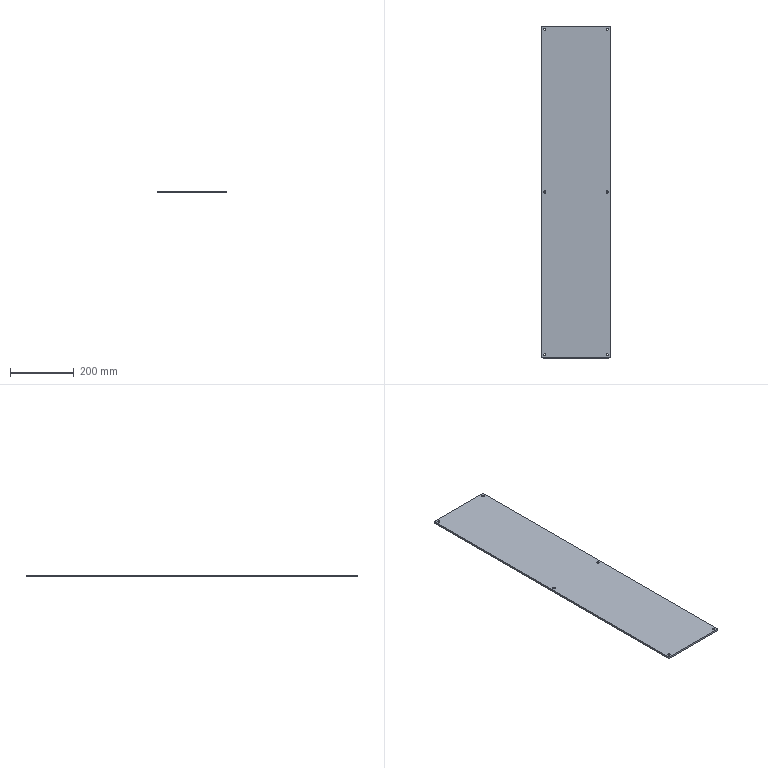Part | SolidWorks | features Extrusion 1, Fillet 1, HoleWzd 1 | 1 solid | 22 faces | box 215 x 1038 x 6 mm | volume 1337506 mm3 | cylinder 16 | plane 6 | commonest cylinder face diameters 7 x12 10 x4
STEP:
#1=CARTESIAN_POINT('',(101.,509.,6.));
#2=VERTEX_POINT('',#1);
#3=CARTESIAN_POINT('',(94.,509.,6.));
#4=VERTEX_POINT('',#3);
#5=CARTESIAN_POINT('',(97.5,509.,6.));
#6=DIRECTION('',(0.,0.,-1.));
#7=DIRECTION('',(-1.,0.,0.));
#8=AXIS2_PLACEMENT_3D('',#5,#6,#7);
#9=CIRCLE('',#8,3.5);
#10=EDGE_CURVE('',#2,#4,#9,.T.);
#11=ORIENTED_EDGE('',*,*,#10,.F.);
#12=CARTESIAN_POINT('',(101.,509.,0.));
#13=VERTEX_POINT('',#12);
#14=CARTESIAN_POINT('',(101.,509.,0.));
#15=DIRECTION('',(0.,0.,-1.));
#16=VECTOR('',#15,1000.);
#17=LINE('',#14,#16);
#18=EDGE_CURVE('',#2,#13,#17,.T.);
#19=ORIENTED_EDGE('',*,*,#18,.T.);
#20=CARTESIAN_POINT('',(94.,509.,0.));
#21=VERTEX_POINT('',#20);
#22=CARTESIAN_POINT('',(97.5,509.,0.));
#23=DIRECTION('',(0.,0.,-1.));
#24=DIRECTION('',(-1.,0.,0.));
#25=AXIS2_PLACEMENT_3D('',#22,#23,#24);
#26=CIRCLE('',#25,3.5);
#27=EDGE_CURVE('',#13,#21,#26,.T.);
#28=ORIENTED_EDGE('',*,*,#27,.T.);
#29=CARTESIAN_POINT('',(94.,509.,0.));
#30=DIRECTION('',(0.,0.,-1.));
#31=VECTOR('',#30,1000.);
#32=LINE('',#29,#31);
#33=EDGE_CURVE('',#4,#21,#32,.T.);
#34=ORIENTED_EDGE('',*,*,#33,.F.);
#35=EDGE_LOOP('',(#11,#19,#28,#34));
#36=FACE_OUTER_BOUND('',#35,.T.);
#37=CARTESIAN_POINT('',(97.5,509.,0.));
#38=DIRECTION('',(0.,0.,-1.));
#39=DIRECTION('',(-1.,0.,0.));
#40=AXIS2_PLACEMENT_3D('',#37,#38,#39);
#41=CYLINDRICAL_SURFACE('',#40,3.5);
#42=ADVANCED_FACE('',(#36),#41,.F.);
#43=CARTESIAN_POINT('',(101.,-509.,6.));
#44=VERTEX_POINT('',#43);
#45=CARTESIAN_POINT('',(94.,-509.,6.));
#46=VERTEX_POINT('',#45);
#47=CARTESIAN_POINT('',(97.5,-509.,6.));
#48=DIRECTION('',(0.,0.,-1.));
#49=DIRECTION('',(-1.,0.,0.));
#50=AXIS2_PLACEMENT_3D('',#47,#48,#49);
#51=CIRCLE('',#50,3.5);
#52=EDGE_CURVE('',#44,#46,#51,.T.);
#53=ORIENTED_EDGE('',*,*,#52,.F.);
#54=CARTESIAN_POINT('',(101.,-509.,0.));
#55=VERTEX_POINT('',#54);
#56=CARTESIAN_POINT('',(101.,-509.,0.));
#57=DIRECTION('',(0.,0.,-1.));
#58=VECTOR('',#57,1000.);
#59=LINE('',#56,#58);
#60=EDGE_CURVE('',#44,#55,#59,.T.);
#61=ORIENTED_EDGE('',*,*,#60,.T.);
#62=CARTESIAN_POINT('',(94.,-509.,0.));
#63=VERTEX_POINT('',#62);
#64=CARTESIAN_POINT('',(97.5,-509.,0.));
#65=DIRECTION('',(0.,0.,-1.));
#66=DIRECTION('',(-1.,0.,0.));
#67=AXIS2_PLACEMENT_3D('',#64,#65,#66);
#68=CIRCLE('',#67,3.5);
#69=EDGE_CURVE('',#55,#63,#68,.T.);
#70=ORIENTED_EDGE('',*,*,#69,.T.);
#71=CARTESIAN_POINT('',(94.,-509.,0.));
#72=DIRECTION('',(0.,0.,-1.));
#73=VECTOR('',#72,1000.);
#74=LINE('',#71,#73);
#75=EDGE_CURVE('',#46,#63,#74,.T.);
#76=ORIENTED_EDGE('',*,*,#75,.F.);
#77=EDGE_LOOP('',(#53,#61,#70,#76));
#78=FACE_OUTER_BOUND('',#77,.T.);
#79=CARTESIAN_POINT('',(97.5,-509.,0.));
#80=DIRECTION('',(0.,0.,-1.));
#81=DIRECTION('',(-1.,0.,0.));
#82=AXIS2_PLACEMENT_3D('',#79,#80,#81);
#83=CYLINDRICAL_SURFACE('',#82,3.5);
#84=ADVANCED_FACE('',(#78),#83,.F.);
#85=CARTESIAN_POINT('',(-94.,509.,6.));
#86=VERTEX_POINT('',#85);
#87=CARTESIAN_POINT('',(-101.,509.,6.));
#88=VERTEX_POINT('',#87);
#89=CARTESIAN_POINT('',(-97.5,509.,6.));
#90=DIRECTION('',(0.,0.,-1.));
#91=DIRECTION('',(-1.,0.,0.));
#92=AXIS2_PLACEMENT_3D('',#89,#90,#91);
#93=CIRCLE('',#92,3.5);
#94=EDGE_CURVE('',#86,#88,#93,.T.);
#95=ORIENTED_EDGE('',*,*,#94,.F.);
#96=CARTESIAN_POINT('',(-94.,509.,0.));
#97=VERTEX_POINT('',#96);
#98=CARTESIAN_POINT('',(-94.,509.,0.));
#99=DIRECTION('',(0.,0.,-1.));
#100=VECTOR('',#99,1000.);
#101=LINE('',#98,#100);
#102=EDGE_CURVE('',#86,#97,#101,.T.);
#103=ORIENTED_EDGE('',*,*,#102,.T.);
#104=CARTESIAN_POINT('',(-101.,509.,0.));
#105=VERTEX_POINT('',#104);
#106=CARTESIAN_POINT('',(-97.5,509.,0.));
#107=DIRECTION('',(0.,0.,-1.));
#108=DIRECTION('',(-1.,0.,0.));
#109=AXIS2_PLACEMENT_3D('',#106,#107,#108);
#110=CIRCLE('',#109,3.5);
#111=EDGE_CURVE('',#97,#105,#110,.T.);
#112=ORIENTED_EDGE('',*,*,#111,.T.);
#113=CARTESIAN_POINT('',(-101.,509.,0.));
#114=DIRECTION('',(0.,0.,-1.));
#115=VECTOR('',#114,1000.);
#116=LINE('',#113,#115);
#117=EDGE_CURVE('',#88,#105,#116,.T.);
#118=ORIENTED_EDGE('',*,*,#117,.F.);
#119=EDGE_LOOP('',(#95,#103,#112,#118));
#120=FACE_OUTER_BOUND('',#119,.T.);
#121=CARTESIAN_POINT('',(-97.5,509.,0.));
#122=DIRECTION('',(0.,0.,-1.));
#123=DIRECTION('',(-1.,0.,0.));
#124=AXIS2_PLACEMENT_3D('',#121,#122,#123);
#125=CYLINDRICAL_SURFACE('',#124,3.5);
#126=ADVANCED_FACE('',(#120),#125,.F.);
#127=CARTESIAN_POINT('',(-94.,-509.,6.));
#128=VERTEX_POINT('',#127);
#129=CARTESIAN_POINT('',(-101.,-509.,6.));
#130=VERTEX_POINT('',#129);
#131=CARTESIAN_POINT('',(-97.5,-509.,6.));
#132=DIRECTION('',(0.,0.,-1.));
#133=DIRECTION('',(-1.,0.,0.));
#134=AXIS2_PLACEMENT_3D('',#131,#132,#133);
#135=CIRCLE('',#134,3.5);
#136=EDGE_CURVE('',#128,#130,#135,.T.);
#137=ORIENTED_EDGE('',*,*,#136,.F.);
#138=CARTESIAN_POINT('',(-94.,-509.,0.));
#139=VERTEX_POINT('',#138);
#140=CARTESIAN_POINT('',(-94.,-509.,0.));
#141=DIRECTION('',(0.,0.,-1.));
#142=VECTOR('',#141,1000.);
#143=LINE('',#140,#142);
#144=EDGE_CURVE('',#128,#139,#143,.T.);
#145=ORIENTED_EDGE('',*,*,#144,.T.);
#146=CARTESIAN_POINT('',(-101.,-509.,0.));
#147=VERTEX_POINT('',#146);
#148=CARTESIAN_POINT('',(-97.5,-509.,0.));
#149=DIRECTION('',(0.,0.,-1.));
#150=DIRECTION('',(-1.,0.,0.));
#151=AXIS2_PLACEMENT_3D('',#148,#149,#150);
#152=CIRCLE('',#151,3.5);
#153=EDGE_CURVE('',#139,#147,#152,.T.);
#154=ORIENTED_EDGE('',*,*,#153,.T.);
#155=CARTESIAN_POINT('',(-101.,-509.,0.));
#156=DIRECTION('',(0.,0.,-1.));
#157=VECTOR('',#156,1000.);
#158=LINE('',#155,#157);
#159=EDGE_CURVE('',#130,#147,#158,.T.);
#160=ORIENTED_EDGE('',*,*,#159,.F.);
#161=EDGE_LOOP('',(#137,#145,#154,#160));
#162=FACE_OUTER_BOUND('',#161,.T.);
#163=CARTESIAN_POINT('',(-97.5,-509.,0.));
#164=DIRECTION('',(0.,0.,-1.));
#165=DIRECTION('',(-1.,0.,0.));
#166=AXIS2_PLACEMENT_3D('',#163,#164,#165);
#167=CYLINDRICAL_SURFACE('',#166,3.5);
#168=ADVANCED_FACE('',(#162),#167,.F.);
#169=CARTESIAN_POINT('',(101.,0.,6.));
#170=VERTEX_POINT('',#169);
#171=CARTESIAN_POINT('',(94.,0.,6.));
#172=VERTEX_POINT('',#171);
#173=CARTESIAN_POINT('',(97.5,0.,6.));
#174=DIRECTION('',(0.,0.,-1.));
#175=DIRECTION('',(-1.,0.,0.));
#176=AXIS2_PLACEMENT_3D('',#173,#174,#175);
#177=CIRCLE('',#176,3.5);
#178=EDGE_CURVE('',#170,#172,#177,.T.);
#179=ORIENTED_EDGE('',*,*,#178,.F.);
#180=CARTESIAN_POINT('',(101.,0.,0.));
#181=VERTEX_POINT('',#180);
#182=CARTESIAN_POINT('',(101.,0.,0.));
#183=DIRECTION('',(0.,0.,-1.));
#184=VECTOR('',#183,1000.);
#185=LINE('',#182,#184);
#186=EDGE_CURVE('',#170,#181,#185,.T.);
#187=ORIENTED_EDGE('',*,*,#186,.T.);
#188=CARTESIAN_POINT('',(94.,0.,0.));
#189=VERTEX_POINT('',#188);
#190=CARTESIAN_POINT('',(97.5,0.,0.));
#191=DIRECTION('',(0.,0.,-1.));
#192=DIRECTION('',(-1.,0.,0.));
#193=AXIS2_PLACEMENT_3D('',#190,#191,#192);
#194=CIRCLE('',#193,3.5);
#195=EDGE_CURVE('',#181,#189,#194,.T.);
#196=ORIENTED_EDGE('',*,*,#195,.T.);
#197=CARTESIAN_POINT('',(94.,0.,0.));
#198=DIRECTION('',(0.,0.,-1.));
#199=VECTOR('',#198,1000.);
#200=LINE('',#197,#199);
#201=EDGE_CURVE('',#172,#189,#200,.T.);
#202=ORIENTED_EDGE('',*,*,#201,.F.);
#203=EDGE_LOOP('',(#179,#187,#196,#202));
#204=FACE_OUTER_BOUND('',#203,.T.);
#205=CARTESIAN_POINT('',(97.5,0.,0.));
#206=DIRECTION('',(0.,0.,-1.));
#207=DIRECTION('',(-1.,0.,0.));
#208=AXIS2_PLACEMENT_3D('',#205,#206,#207);
#209=CYLINDRICAL_SURFACE('',#208,3.5);
#210=ADVANCED_FACE('',(#204),#209,.F.);
#211=CARTESIAN_POINT('',(-94.,0.,6.));
#212=VERTEX_POINT('',#211);
#213=CARTESIAN_POINT('',(-101.,0.,6.));
#214=VERTEX_POINT('',#213);
#215=CARTESIAN_POINT('',(-97.5,0.,6.));
#216=DIRECTION('',(0.,0.,-1.));
#217=DIRECTION('',(-1.,0.,0.));
#218=AXIS2_PLACEMENT_3D('',#215,#216,#217);
#219=CIRCLE('',#218,3.5);
#220=EDGE_CURVE('',#212,#214,#219,.T.);
#221=ORIENTED_EDGE('',*,*,#220,.F.);
#222=CARTESIAN_POINT('',(-94.,0.,0.));
#223=VERTEX_POINT('',#222);
#224=CARTESIAN_POINT('',(-94.,0.,0.));
#225=DIRECTION('',(0.,0.,-1.));
#226=VECTOR('',#225,1000.);
#227=LINE('',#224,#226);
#228=EDGE_CURVE('',#212,#223,#227,.T.);
#229=ORIENTED_EDGE('',*,*,#228,.T.);
#230=CARTESIAN_POINT('',(-101.,0.,0.));
#231=VERTEX_POINT('',#230);
#232=CARTESIAN_POINT('',(-97.5,0.,0.));
#233=DIRECTION('',(0.,0.,-1.));
#234=DIRECTION('',(-1.,0.,0.));
#235=AXIS2_PLACEMENT_3D('',#232,#233,#234);
#236=CIRCLE('',#235,3.5);
#237=EDGE_CURVE('',#223,#231,#236,.T.);
#238=ORIENTED_EDGE('',*,*,#237,.T.);
#239=CARTESIAN_POINT('',(-101.,0.,0.));
#240=DIRECTION('',(0.,0.,-1.));
#241=VECTOR('',#240,1000.);
#242=LINE('',#239,#241);
#243=EDGE_CURVE('',#214,#231,#242,.T.);
#244=ORIENTED_EDGE('',*,*,#243,.F.);
#245=EDGE_LOOP('',(#221,#229,#238,#244));
#246=FACE_OUTER_BOUND('',#245,.T.);
#247=CARTESIAN_POINT('',(-97.5,0.,0.));
#248=DIRECTION('',(0.,0.,-1.));
#249=DIRECTION('',(-1.,0.,0.));
#250=AXIS2_PLACEMENT_3D('',#247,#248,#249);
#251=CYLINDRICAL_SURFACE('',#250,3.5);
#252=ADVANCED_FACE('',(#246),#251,.F.);
#253=CARTESIAN_POINT('',(107.5,-514.,6.));
#254=VERTEX_POINT('',#253);
#255=CARTESIAN_POINT('',(107.5,514.,6.));
#256=VERTEX_POINT('',#255);
#257=CARTESIAN_POINT('',(107.5,519.,6.));
#258=DIRECTION('',(0.,1.,0.));
#259=VECTOR('',#258,1000.);
#260=LINE('',#257,#259);
#261=EDGE_CURVE('',#254,#256,#260,.T.);
#262=ORIENTED_EDGE('',*,*,#261,.F.);
#263=CARTESIAN_POINT('',(107.5,-514.,0.));
#264=VERTEX_POINT('',#263);
#265=CARTESIAN_POINT('',(107.5,-514.,6.));
#266=DIRECTION('',(0.,0.,-1.));
#267=VECTOR('',#266,1000.);
#268=LINE('',#265,#267);
#269=EDGE_CURVE('',#254,#264,#268,.T.);
#270=ORIENTED_EDGE('',*,*,#269,.T.);
#271=CARTESIAN_POINT('',(107.5,514.,0.));
#272=VERTEX_POINT('',#271);
#273=CARTESIAN_POINT('',(107.5,519.,0.));
#274=DIRECTION('',(0.,1.,0.));
#275=VECTOR('',#274,1000.);
#276=LINE('',#273,#275);
#277=EDGE_CURVE('',#264,#272,#276,.T.);
#278=ORIENTED_EDGE('',*,*,#277,.T.);
#279=CARTESIAN_POINT('',(107.5,514.,6.));
#280=DIRECTION('',(0.,0.,1.));
#281=VECTOR('',#280,1000.);
#282=LINE('',#279,#281);
#283=EDGE_CURVE('',#272,#256,#282,.T.);
#284=ORIENTED_EDGE('',*,*,#283,.T.);
#285=EDGE_LOOP('',(#262,#270,#278,#284));
#286=FACE_OUTER_BOUND('',#285,.T.);
#287=CARTESIAN_POINT('',(107.5,519.,6.));
#288=DIRECTION('',(-1.,0.,0.));
#289=DIRECTION('',(0.,-1.,0.));
#290=AXIS2_PLACEMENT_3D('',#287,#288,#289);
#291=PLANE('',#290);
#292=ADVANCED_FACE('',(#286),#291,.F.);
#293=CARTESIAN_POINT('',(102.5,519.,0.));
#294=VERTEX_POINT('',#293);
#295=CARTESIAN_POINT('',(-102.5,519.,0.));
#296=VERTEX_POINT('',#295);
#297=CARTESIAN_POINT('',(-107.5,519.,0.));
#298=DIRECTION('',(-1.,0.,0.));
#299=VECTOR('',#298,1000.);
#300=LINE('',#297,#299);
#301=EDGE_CURVE('',#294,#296,#300,.T.);
#302=ORIENTED_EDGE('',*,*,#301,.T.);
#303=CARTESIAN_POINT('',(-102.5,519.,6.));
#304=VERTEX_POINT('',#303);
#305=CARTESIAN_POINT('',(-102.5,519.,6.));
#306=DIRECTION('',(0.,0.,1.));
#307=VECTOR('',#306,1000.);
#308=LINE('',#305,#307);
#309=EDGE_CURVE('',#296,#304,#308,.T.);
#310=ORIENTED_EDGE('',*,*,#309,.T.);
#311=CARTESIAN_POINT('',(102.5,519.,6.));
#312=VERTEX_POINT('',#311);
#313=CARTESIAN_POINT('',(-107.5,519.,6.));
#314=DIRECTION('',(-1.,0.,0.));
#315=VECTOR('',#314,1000.);
#316=LINE('',#313,#315);
#317=EDGE_CURVE('',#312,#304,#316,.T.);
#318=ORIENTED_EDGE('',*,*,#317,.F.);
#319=CARTESIAN_POINT('',(102.5,519.,6.));
#320=DIRECTION('',(0.,0.,-1.));
#321=VECTOR('',#320,1000.);
#322=LINE('',#319,#321);
#323=EDGE_CURVE('',#312,#294,#322,.T.);
#324=ORIENTED_EDGE('',*,*,#323,.T.);
#325=EDGE_LOOP('',(#302,#310,#318,#324));
#326=FACE_OUTER_BOUND('',#325,.T.);
#327=CARTESIAN_POINT('',(-107.5,519.,6.));
#328=DIRECTION('',(0.,-1.,0.));
#329=DIRECTION('',(0.,0.,-1.));
#330=AXIS2_PLACEMENT_3D('',#327,#328,#329);
#331=PLANE('',#330);
#332=ADVANCED_FACE('',(#326),#331,.F.);
#333=CARTESIAN_POINT('',(-107.5,514.,0.));
#334=VERTEX_POINT('',#333);
#335=CARTESIAN_POINT('',(-107.5,-514.,0.));
#336=VERTEX_POINT('',#335);
#337=CARTESIAN_POINT('',(-107.5,519.,0.));
#338=DIRECTION('',(0.,-1.,0.));
#339=VECTOR('',#338,1000.);
#340=LINE('',#337,#339);
#341=EDGE_CURVE('',#334,#336,#340,.T.);
#342=ORIENTED_EDGE('',*,*,#341,.T.);
#343=CARTESIAN_POINT('',(-107.5,-514.,6.));
#344=VERTEX_POINT('',#343);
#345=CARTESIAN_POINT('',(-107.5,-514.,6.));
#346=DIRECTION('',(0.,0.,1.));
#347=VECTOR('',#346,1000.);
#348=LINE('',#345,#347);
#349=EDGE_CURVE('',#336,#344,#348,.T.);
#350=ORIENTED_EDGE('',*,*,#349,.T.);
#351=CARTESIAN_POINT('',(-107.5,514.,6.));
#352=VERTEX_POINT('',#351);
#353=CARTESIAN_POINT('',(-107.5,519.,6.));
#354=DIRECTION('',(0.,-1.,0.));
#355=VECTOR('',#354,1000.);
#356=LINE('',#353,#355);
#357=EDGE_CURVE('',#352,#344,#356,.T.);
#358=ORIENTED_EDGE('',*,*,#357,.F.);
#359=CARTESIAN_POINT('',(-107.5,514.,6.));
#360=DIRECTION('',(0.,0.,-1.));
#361=VECTOR('',#360,1000.);
#362=LINE('',#359,#361);
#363=EDGE_CURVE('',#352,#334,#362,.T.);
#364=ORIENTED_EDGE('',*,*,#363,.T.);
#365=EDGE_LOOP('',(#342,#350,#358,#364));
#366=FACE_OUTER_BOUND('',#365,.T.);
#367=CARTESIAN_POINT('',(-107.5,519.,6.));
#368=DIRECTION('',(1.,0.,0.));
#369=DIRECTION('',(0.,1.,0.));
#370=AXIS2_PLACEMENT_3D('',#367,#368,#369);
#371=PLANE('',#370);
#372=ADVANCED_FACE('',(#366),#371,.F.);
#373=CARTESIAN_POINT('',(-102.5,-519.,6.));
#374=VERTEX_POINT('',#373);
#375=CARTESIAN_POINT('',(102.5,-519.,6.));
#376=VERTEX_POINT('',#375);
#377=CARTESIAN_POINT('',(-107.5,-519.,6.));
#378=DIRECTION('',(1.,0.,0.));
#379=VECTOR('',#378,1000.);
#380=LINE('',#377,#379);
#381=EDGE_CURVE('',#374,#376,#380,.T.);
#382=ORIENTED_EDGE('',*,*,#381,.F.);
#383=CARTESIAN_POINT('',(-102.5,-519.,0.));
#384=VERTEX_POINT('',#383);
#385=CARTESIAN_POINT('',(-102.5,-519.,6.));
#386=DIRECTION('',(0.,0.,-1.));
#387=VECTOR('',#386,1000.);
#388=LINE('',#385,#387);
#389=EDGE_CURVE('',#374,#384,#388,.T.);
#390=ORIENTED_EDGE('',*,*,#389,.T.);
#391=CARTESIAN_POINT('',(102.5,-519.,0.));
#392=VERTEX_POINT('',#391);
#393=CARTESIAN_POINT('',(-107.5,-519.,0.));
#394=DIRECTION('',(1.,0.,0.));
#395=VECTOR('',#394,1000.);
#396=LINE('',#393,#395);
#397=EDGE_CURVE('',#384,#392,#396,.T.);
#398=ORIENTED_EDGE('',*,*,#397,.T.);
#399=CARTESIAN_POINT('',(102.5,-519.,6.));
#400=DIRECTION('',(0.,0.,1.));
#401=VECTOR('',#400,1000.);
#402=LINE('',#399,#401);
#403=EDGE_CURVE('',#392,#376,#402,.T.);
#404=ORIENTED_EDGE('',*,*,#403,.T.);
#405=EDGE_LOOP('',(#382,#390,#398,#404));
#406=FACE_OUTER_BOUND('',#405,.T.);
#407=CARTESIAN_POINT('',(-107.5,-519.,6.));
#408=DIRECTION('',(0.,1.,0.));
#409=DIRECTION('',(0.,0.,1.));
#410=AXIS2_PLACEMENT_3D('',#407,#408,#409);
#411=PLANE('',#410);
#412=ADVANCED_FACE('',(#406),#411,.F.);
#413=CARTESIAN_POINT('',(97.5,509.,6.));
#414=DIRECTION('',(0.,0.,-1.));
#415=DIRECTION('',(-1.,0.,0.));
#416=AXIS2_PLACEMENT_3D('',#413,#414,#415);
#417=CIRCLE('',#416,3.5);
#418=EDGE_CURVE('',#4,#2,#417,.T.);
#419=ORIENTED_EDGE('',*,*,#418,.T.);
#420=ORIENTED_EDGE('',*,*,#10,.T.);
#421=EDGE_LOOP('',(#419,#420));
#422=FACE_BOUND('',#421,.T.);
#423=CARTESIAN_POINT('',(97.5,-509.,6.));
#424=DIRECTION('',(0.,0.,-1.));
#425=DIRECTION('',(-1.,0.,0.));
#426=AXIS2_PLACEMENT_3D('',#423,#424,#425);
#427=CIRCLE('',#426,3.5);
#428=EDGE_CURVE('',#46,#44,#427,.T.);
#429=ORIENTED_EDGE('',*,*,#428,.T.);
#430=ORIENTED_EDGE('',*,*,#52,.T.);
#431=EDGE_LOOP('',(#429,#430));
#432=FACE_BOUND('',#431,.T.);
#433=CARTESIAN_POINT('',(-97.5,509.,6.));
#434=DIRECTION('',(0.,0.,-1.));
#435=DIRECTION('',(-1.,0.,0.));
#436=AXIS2_PLACEMENT_3D('',#433,#434,#435);
#437=CIRCLE('',#436,3.5);
#438=EDGE_CURVE('',#88,#86,#437,.T.);
#439=ORIENTED_EDGE('',*,*,#438,.T.);
#440=ORIENTED_EDGE('',*,*,#94,.T.);
#441=EDGE_LOOP('',(#439,#440));
#442=FACE_BOUND('',#441,.T.);
#443=CARTESIAN_POINT('',(-97.5,-509.,6.));
#444=DIRECTION('',(0.,0.,-1.));
#445=DIRECTION('',(-1.,0.,0.));
#446=AXIS2_PLACEMENT_3D('',#443,#444,#445);
#447=CIRCLE('',#446,3.5);
#448=EDGE_CURVE('',#130,#128,#447,.T.);
#449=ORIENTED_EDGE('',*,*,#448,.T.);
#450=ORIENTED_EDGE('',*,*,#136,.T.);
#451=EDGE_LOOP('',(#449,#450));
#452=FACE_BOUND('',#451,.T.);
#453=CARTESIAN_POINT('',(97.5,0.,6.));
#454=DIRECTION('',(0.,0.,-1.));
#455=DIRECTION('',(-1.,0.,0.));
#456=AXIS2_PLACEMENT_3D('',#453,#454,#455);
#457=CIRCLE('',#456,3.5);
#458=EDGE_CURVE('',#172,#170,#457,.T.);
#459=ORIENTED_EDGE('',*,*,#458,.T.);
#460=ORIENTED_EDGE('',*,*,#178,.T.);
#461=EDGE_LOOP('',(#459,#460));
#462=FACE_BOUND('',#461,.T.);
#463=CARTESIAN_POINT('',(-97.5,0.,6.));
#464=DIRECTION('',(0.,0.,-1.));
#465=DIRECTION('',(-1.,0.,0.));
#466=AXIS2_PLACEMENT_3D('',#463,#464,#465);
#467=CIRCLE('',#466,3.5);
#468=EDGE_CURVE('',#214,#212,#467,.T.);
#469=ORIENTED_EDGE('',*,*,#468,.T.);
#470=ORIENTED_EDGE('',*,*,#220,.T.);
#471=EDGE_LOOP('',(#469,#470));
#472=FACE_BOUND('',#471,.T.);
#473=ORIENTED_EDGE('',*,*,#357,.T.);
#474=CARTESIAN_POINT('',(-102.5,-514.,6.));
#475=DIRECTION('',(0.,0.,1.));
#476=DIRECTION('',(1.,0.,0.));
#477=AXIS2_PLACEMENT_3D('',#474,#475,#476);
#478=CIRCLE('',#477,5.);
#479=EDGE_CURVE('',#344,#374,#478,.T.);
#480=ORIENTED_EDGE('',*,*,#479,.T.);
#481=ORIENTED_EDGE('',*,*,#381,.T.);
#482=CARTESIAN_POINT('',(102.5,-514.,6.));
#483=DIRECTION('',(0.,0.,1.));
#484=DIRECTION('',(1.,0.,0.));
#485=AXIS2_PLACEMENT_3D('',#482,#483,#484);
#486=CIRCLE('',#485,5.);
#487=EDGE_CURVE('',#376,#254,#486,.T.);
#488=ORIENTED_EDGE('',*,*,#487,.T.);
#489=ORIENTED_EDGE('',*,*,#261,.T.);
#490=CARTESIAN_POINT('',(102.5,514.,6.));
#491=DIRECTION('',(0.,0.,1.));
#492=DIRECTION('',(1.,0.,0.));
#493=AXIS2_PLACEMENT_3D('',#490,#491,#492);
#494=CIRCLE('',#493,5.);
#495=EDGE_CURVE('',#256,#312,#494,.T.);
#496=ORIENTED_EDGE('',*,*,#495,.T.);
#497=ORIENTED_EDGE('',*,*,#317,.T.);
#498=CARTESIAN_POINT('',(-102.5,514.,6.));
#499=DIRECTION('',(0.,0.,1.));
#500=DIRECTION('',(1.,0.,0.));
#501=AXIS2_PLACEMENT_3D('',#498,#499,#500);
#502=CIRCLE('',#501,5.);
#503=EDGE_CURVE('',#304,#352,#502,.T.);
#504=ORIENTED_EDGE('',*,*,#503,.T.);
#505=EDGE_LOOP('',(#473,#480,#481,#488,#489,#496,#497,#504));
#506=FACE_OUTER_BOUND('',#505,.T.);
#507=CARTESIAN_POINT('',(0.,0.,6.));
#508=DIRECTION('',(0.,0.,1.));
#509=DIRECTION('',(1.,0.,0.));
#510=AXIS2_PLACEMENT_3D('',#507,#508,#509);
#511=PLANE('',#510);
#512=ADVANCED_FACE('',(#422,#432,#442,#452,#462,#472,#506),#511,.T.);
#513=CARTESIAN_POINT('',(97.5,509.,0.));
#514=DIRECTION('',(0.,0.,-1.));
#515=DIRECTION('',(-1.,0.,0.));
#516=AXIS2_PLACEMENT_3D('',#513,#514,#515);
#517=CIRCLE('',#516,3.5);
#518=EDGE_CURVE('',#21,#13,#517,.T.);
#519=ORIENTED_EDGE('',*,*,#518,.F.);
#520=ORIENTED_EDGE('',*,*,#27,.F.);
#521=EDGE_LOOP('',(#519,#520));
#522=FACE_BOUND('',#521,.T.);
#523=CARTESIAN_POINT('',(97.5,-509.,0.));
#524=DIRECTION('',(0.,0.,-1.));
#525=DIRECTION('',(-1.,0.,0.));
#526=AXIS2_PLACEMENT_3D('',#523,#524,#525);
#527=CIRCLE('',#526,3.5);
#528=EDGE_CURVE('',#63,#55,#527,.T.);
#529=ORIENTED_EDGE('',*,*,#528,.F.);
#530=ORIENTED_EDGE('',*,*,#69,.F.);
#531=EDGE_LOOP('',(#529,#530));
#532=FACE_BOUND('',#531,.T.);
#533=CARTESIAN_POINT('',(-97.5,509.,0.));
#534=DIRECTION('',(0.,0.,-1.));
#535=DIRECTION('',(-1.,0.,0.));
#536=AXIS2_PLACEMENT_3D('',#533,#534,#535);
#537=CIRCLE('',#536,3.5);
#538=EDGE_CURVE('',#105,#97,#537,.T.);
#539=ORIENTED_EDGE('',*,*,#538,.F.);
#540=ORIENTED_EDGE('',*,*,#111,.F.);
#541=EDGE_LOOP('',(#539,#540));
#542=FACE_BOUND('',#541,.T.);
#543=CARTESIAN_POINT('',(-97.5,-509.,0.));
#544=DIRECTION('',(0.,0.,-1.));
#545=DIRECTION('',(-1.,0.,0.));
#546=AXIS2_PLACEMENT_3D('',#543,#544,#545);
#547=CIRCLE('',#546,3.5);
#548=EDGE_CURVE('',#147,#139,#547,.T.);
#549=ORIENTED_EDGE('',*,*,#548,.F.);
#550=ORIENTED_EDGE('',*,*,#153,.F.);
#551=EDGE_LOOP('',(#549,#550));
#552=FACE_BOUND('',#551,.T.);
#553=CARTESIAN_POINT('',(97.5,0.,0.));
#554=DIRECTION('',(0.,0.,-1.));
#555=DIRECTION('',(-1.,0.,0.));
#556=AXIS2_PLACEMENT_3D('',#553,#554,#555);
#557=CIRCLE('',#556,3.5);
#558=EDGE_CURVE('',#189,#181,#557,.T.);
#559=ORIENTED_EDGE('',*,*,#558,.F.);
#560=ORIENTED_EDGE('',*,*,#195,.F.);
#561=EDGE_LOOP('',(#559,#560));
#562=FACE_BOUND('',#561,.T.);
#563=CARTESIAN_POINT('',(-97.5,0.,0.));
#564=DIRECTION('',(0.,0.,-1.));
#565=DIRECTION('',(-1.,0.,0.));
#566=AXIS2_PLACEMENT_3D('',#563,#564,#565);
#567=CIRCLE('',#566,3.5);
#568=EDGE_CURVE('',#231,#223,#567,.T.);
#569=ORIENTED_EDGE('',*,*,#568,.F.);
#570=ORIENTED_EDGE('',*,*,#237,.F.);
#571=EDGE_LOOP('',(#569,#570));
#572=FACE_BOUND('',#571,.T.);
#573=ORIENTED_EDGE('',*,*,#397,.F.);
#574=CARTESIAN_POINT('',(-102.5,-514.,0.));
#575=DIRECTION('',(0.,0.,-1.));
#576=DIRECTION('',(1.,0.,0.));
#577=AXIS2_PLACEMENT_3D('',#574,#575,#576);
#578=CIRCLE('',#577,5.);
#579=EDGE_CURVE('',#384,#336,#578,.T.);
#580=ORIENTED_EDGE('',*,*,#579,.T.);
#581=ORIENTED_EDGE('',*,*,#341,.F.);
#582=CARTESIAN_POINT('',(-102.5,514.,0.));
#583=DIRECTION('',(0.,0.,-1.));
#584=DIRECTION('',(1.,0.,0.));
#585=AXIS2_PLACEMENT_3D('',#582,#583,#584);
#586=CIRCLE('',#585,5.);
#587=EDGE_CURVE('',#334,#296,#586,.T.);
#588=ORIENTED_EDGE('',*,*,#587,.T.);
#589=ORIENTED_EDGE('',*,*,#301,.F.);
#590=CARTESIAN_POINT('',(102.5,514.,0.));
#591=DIRECTION('',(0.,0.,-1.));
#592=DIRECTION('',(1.,0.,0.));
#593=AXIS2_PLACEMENT_3D('',#590,#591,#592);
#594=CIRCLE('',#593,5.);
#595=EDGE_CURVE('',#294,#272,#594,.T.);
#596=ORIENTED_EDGE('',*,*,#595,.T.);
#597=ORIENTED_EDGE('',*,*,#277,.F.);
#598=CARTESIAN_POINT('',(102.5,-514.,0.));
#599=DIRECTION('',(0.,0.,-1.));
#600=DIRECTION('',(1.,0.,0.));
#601=AXIS2_PLACEMENT_3D('',#598,#599,#600);
#602=CIRCLE('',#601,5.);
#603=EDGE_CURVE('',#264,#392,#602,.T.);
#604=ORIENTED_EDGE('',*,*,#603,.T.);
#605=EDGE_LOOP('',(#573,#580,#581,#588,#589,#596,#597,#604));
#606=FACE_OUTER_BOUND('',#605,.T.);
#607=CARTESIAN_POINT('',(0.,0.,0.));
#608=DIRECTION('',(0.,0.,1.));
#609=DIRECTION('',(1.,0.,0.));
#610=AXIS2_PLACEMENT_3D('',#607,#608,#609);
#611=PLANE('',#610);
#612=ADVANCED_FACE('',(#522,#532,#542,#552,#562,#572,#606),#611,.F.);
#613=ORIENTED_EDGE('',*,*,#228,.F.);
#614=ORIENTED_EDGE('',*,*,#468,.F.);
#615=ORIENTED_EDGE('',*,*,#243,.T.);
#616=ORIENTED_EDGE('',*,*,#568,.T.);
#617=EDGE_LOOP('',(#613,#614,#615,#616));
#618=FACE_OUTER_BOUND('',#617,.T.);
#619=CARTESIAN_POINT('',(-97.5,0.,0.));
#620=DIRECTION('',(0.,0.,-1.));
#621=DIRECTION('',(-1.,0.,0.));
#622=AXIS2_PLACEMENT_3D('',#619,#620,#621);
#623=CYLINDRICAL_SURFACE('',#622,3.5);
#624=ADVANCED_FACE('',(#618),#623,.F.);
#625=ORIENTED_EDGE('',*,*,#186,.F.);
#626=ORIENTED_EDGE('',*,*,#458,.F.);
#627=ORIENTED_EDGE('',*,*,#201,.T.);
#628=ORIENTED_EDGE('',*,*,#558,.T.);
#629=EDGE_LOOP('',(#625,#626,#627,#628));
#630=FACE_OUTER_BOUND('',#629,.T.);
#631=CARTESIAN_POINT('',(97.5,0.,0.));
#632=DIRECTION('',(0.,0.,-1.));
#633=DIRECTION('',(-1.,0.,0.));
#634=AXIS2_PLACEMENT_3D('',#631,#632,#633);
#635=CYLINDRICAL_SURFACE('',#634,3.5);
#636=ADVANCED_FACE('',(#630),#635,.F.);
#637=ORIENTED_EDGE('',*,*,#144,.F.);
#638=ORIENTED_EDGE('',*,*,#448,.F.);
#639=ORIENTED_EDGE('',*,*,#159,.T.);
#640=ORIENTED_EDGE('',*,*,#548,.T.);
#641=EDGE_LOOP('',(#637,#638,#639,#640));
#642=FACE_OUTER_BOUND('',#641,.T.);
#643=CARTESIAN_POINT('',(-97.5,-509.,0.));
#644=DIRECTION('',(0.,0.,-1.));
#645=DIRECTION('',(-1.,0.,0.));
#646=AXIS2_PLACEMENT_3D('',#643,#644,#645);
#647=CYLINDRICAL_SURFACE('',#646,3.5);
#648=ADVANCED_FACE('',(#642),#647,.F.);
#649=ORIENTED_EDGE('',*,*,#102,.F.);
#650=ORIENTED_EDGE('',*,*,#438,.F.);
#651=ORIENTED_EDGE('',*,*,#117,.T.);
#652=ORIENTED_EDGE('',*,*,#538,.T.);
#653=EDGE_LOOP('',(#649,#650,#651,#652));
#654=FACE_OUTER_BOUND('',#653,.T.);
#655=CARTESIAN_POINT('',(-97.5,509.,0.));
#656=DIRECTION('',(0.,0.,-1.));
#657=DIRECTION('',(-1.,0.,0.));
#658=AXIS2_PLACEMENT_3D('',#655,#656,#657);
#659=CYLINDRICAL_SURFACE('',#658,3.5);
#660=ADVANCED_FACE('',(#654),#659,.F.);
#661=ORIENTED_EDGE('',*,*,#60,.F.);
#662=ORIENTED_EDGE('',*,*,#428,.F.);
#663=ORIENTED_EDGE('',*,*,#75,.T.);
#664=ORIENTED_EDGE('',*,*,#528,.T.);
#665=EDGE_LOOP('',(#661,#662,#663,#664));
#666=FACE_OUTER_BOUND('',#665,.T.);
#667=CARTESIAN_POINT('',(97.5,-509.,0.));
#668=DIRECTION('',(0.,0.,-1.));
#669=DIRECTION('',(-1.,0.,0.));
#670=AXIS2_PLACEMENT_3D('',#667,#668,#669);
#671=CYLINDRICAL_SURFACE('',#670,3.5);
#672=ADVANCED_FACE('',(#666),#671,.F.);
#673=ORIENTED_EDGE('',*,*,#18,.F.);
#674=ORIENTED_EDGE('',*,*,#418,.F.);
#675=ORIENTED_EDGE('',*,*,#33,.T.);
#676=ORIENTED_EDGE('',*,*,#518,.T.);
#677=EDGE_LOOP('',(#673,#674,#675,#676));
#678=FACE_OUTER_BOUND('',#677,.T.);
#679=CARTESIAN_POINT('',(97.5,509.,0.));
#680=DIRECTION('',(0.,0.,-1.));
#681=DIRECTION('',(-1.,0.,0.));
#682=AXIS2_PLACEMENT_3D('',#679,#680,#681);
#683=CYLINDRICAL_SURFACE('',#682,3.5);
#684=ADVANCED_FACE('',(#678),#683,.F.);
#685=ORIENTED_EDGE('',*,*,#479,.F.);
#686=ORIENTED_EDGE('',*,*,#349,.F.);
#687=ORIENTED_EDGE('',*,*,#579,.F.);
#688=ORIENTED_EDGE('',*,*,#389,.F.);
#689=EDGE_LOOP('',(#685,#686,#687,#688));
#690=FACE_OUTER_BOUND('',#689,.T.);
#691=CARTESIAN_POINT('',(-102.5,-514.,6.));
#692=DIRECTION('',(0.,0.,-1.));
#693=DIRECTION('',(-1.,0.,0.));
#694=AXIS2_PLACEMENT_3D('',#691,#692,#693);
#695=CYLINDRICAL_SURFACE('',#694,5.);
#696=ADVANCED_FACE('',(#690),#695,.T.);
#697=ORIENTED_EDGE('',*,*,#503,.F.);
#698=ORIENTED_EDGE('',*,*,#309,.F.);
#699=ORIENTED_EDGE('',*,*,#587,.F.);
#700=ORIENTED_EDGE('',*,*,#363,.F.);
#701=EDGE_LOOP('',(#697,#698,#699,#700));
#702=FACE_OUTER_BOUND('',#701,.T.);
#703=CARTESIAN_POINT('',(-102.5,514.,6.));
#704=DIRECTION('',(0.,0.,-1.));
#705=DIRECTION('',(-1.,0.,0.));
#706=AXIS2_PLACEMENT_3D('',#703,#704,#705);
#707=CYLINDRICAL_SURFACE('',#706,5.);
#708=ADVANCED_FACE('',(#702),#707,.T.);
#709=ORIENTED_EDGE('',*,*,#487,.F.);
#710=ORIENTED_EDGE('',*,*,#403,.F.);
#711=ORIENTED_EDGE('',*,*,#603,.F.);
#712=ORIENTED_EDGE('',*,*,#269,.F.);
#713=EDGE_LOOP('',(#709,#710,#711,#712));
#714=FACE_OUTER_BOUND('',#713,.T.);
#715=CARTESIAN_POINT('',(102.5,-514.,6.));
#716=DIRECTION('',(0.,0.,-1.));
#717=DIRECTION('',(-1.,0.,0.));
#718=AXIS2_PLACEMENT_3D('',#715,#716,#717);
#719=CYLINDRICAL_SURFACE('',#718,5.);
#720=ADVANCED_FACE('',(#714),#719,.T.);
#721=ORIENTED_EDGE('',*,*,#495,.F.);
#722=ORIENTED_EDGE('',*,*,#283,.F.);
#723=ORIENTED_EDGE('',*,*,#595,.F.);
#724=ORIENTED_EDGE('',*,*,#323,.F.);
#725=EDGE_LOOP('',(#721,#722,#723,#724));
#726=FACE_OUTER_BOUND('',#725,.T.);
#727=CARTESIAN_POINT('',(102.5,514.,6.));
#728=DIRECTION('',(0.,0.,-1.));
#729=DIRECTION('',(-1.,0.,0.));
#730=AXIS2_PLACEMENT_3D('',#727,#728,#729);
#731=CYLINDRICAL_SURFACE('',#730,5.);
#732=ADVANCED_FACE('',(#726),#731,.T.);
#733=CLOSED_SHELL('',(#42,#84,#126,#168,#210,#252,#292,#332,#372,#412,#512,#612,#624,#636,#648,#660,#672,#684,#696,#708,#720,#732));
#734=MANIFOLD_SOLID_BREP('',#733);
#735=CARTESIAN_POINT('',(0.,0.,0.));
#736=DIRECTION('',(0.,0.,1.));
#737=DIRECTION('',(1.,0.,0.));
#738=AXIS2_PLACEMENT_3D('',#735,#736,#737);
#739=(LENGTH_UNIT()NAMED_UNIT(*)SI_UNIT(.MILLI.,.METRE.));
#740=UNCERTAINTY_MEASURE_WITH_UNIT(LENGTH_MEASURE(0.00001),#739,'','');
#741=(NAMED_UNIT(*)PLANE_ANGLE_UNIT()SI_UNIT($,.RADIAN.));
#742=(NAMED_UNIT(*)SI_UNIT($,.STERADIAN.)SOLID_ANGLE_UNIT());
#743=(GEOMETRIC_REPRESENTATION_CONTEXT(3)GLOBAL_UNCERTAINTY_ASSIGNED_CONTEXT((#740))GLOBAL_UNIT_ASSIGNED_CONTEXT((#739,#741,#742))REPRESENTATION_CONTEXT('',''));
#744=ADVANCED_BREP_SHAPE_REPRESENTATION('',(#734,#738),#743);